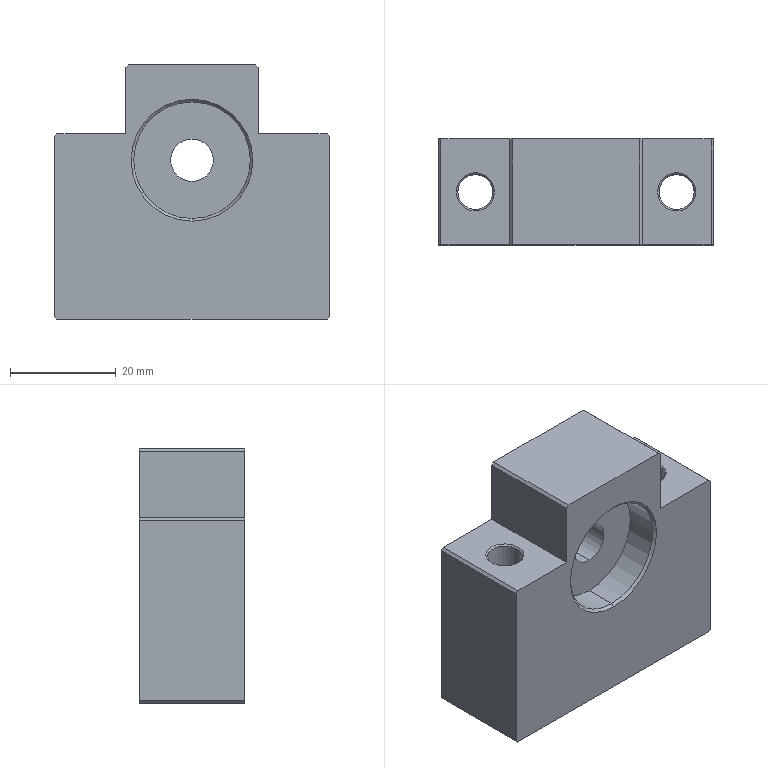Part | SolidWorks | features BaseBody 1 | 1 solid | 36 faces | box 52 x 20 x 48 mm | volume 35177 mm3 | plane 18 | cylinder 10 | cone 8 | commonest cylinder face diameters 6.6 x4 22 x4 8 x2
STEP:
#1=CARTESIAN_POINT('',(290.547,1555.464,-1167.57));
#2=VERTEX_POINT('',#1);
#3=CARTESIAN_POINT('',(290.547,1555.464,-1189.57));
#4=VERTEX_POINT('',#3);
#5=CARTESIAN_POINT('',(290.547,1555.464,-1178.57));
#6=DIRECTION('',(0.,-1.,0.));
#7=DIRECTION('',(1.,0.,0.));
#8=AXIS2_PLACEMENT_3D('',#5,#6,#7);
#9=CIRCLE('',#8,11.);
#10=EDGE_CURVE('',#2,#4,#9,.T.);
#11=ORIENTED_EDGE('',*,*,#10,.F.);
#12=CARTESIAN_POINT('',(290.547,1554.964,-1167.07));
#13=VERTEX_POINT('',#12);
#14=CARTESIAN_POINT('',(290.547,1554.964,-1167.07));
#15=DIRECTION('',(0.,-0.7071,0.7071));
#16=VECTOR('',#15,1000.);
#17=LINE('',#14,#16);
#18=EDGE_CURVE('',#2,#13,#17,.T.);
#19=ORIENTED_EDGE('',*,*,#18,.T.);
#20=CARTESIAN_POINT('',(290.547,1554.964,-1190.07));
#21=VERTEX_POINT('',#20);
#22=CARTESIAN_POINT('',(290.547,1554.964,-1178.57));
#23=DIRECTION('',(0.,-1.,0.));
#24=DIRECTION('',(0.,0.,-1.));
#25=AXIS2_PLACEMENT_3D('',#22,#23,#24);
#26=CIRCLE('',#25,11.5);
#27=EDGE_CURVE('',#13,#21,#26,.T.);
#28=ORIENTED_EDGE('',*,*,#27,.T.);
#29=CARTESIAN_POINT('',(290.547,1554.964,-1190.07));
#30=DIRECTION('',(0.,-0.7071,-0.7071));
#31=VECTOR('',#30,1000.);
#32=LINE('',#29,#31);
#33=EDGE_CURVE('',#4,#21,#32,.T.);
#34=ORIENTED_EDGE('',*,*,#33,.F.);
#35=EDGE_LOOP('',(#11,#19,#28,#34));
#36=FACE_OUTER_BOUND('',#35,.T.);
#37=CARTESIAN_POINT('',(290.547,1554.964,-1178.57));
#38=DIRECTION('',(0.,-1.,0.));
#39=DIRECTION('',(0.,0.,-1.));
#40=AXIS2_PLACEMENT_3D('',#37,#38,#39);
#41=CONICAL_SURFACE('',#40,11.5,0.7854);
#42=ADVANCED_FACE('',(#36),#41,.F.);
#43=ORIENTED_EDGE('',*,*,#10,.T.);
#44=CARTESIAN_POINT('',(290.547,1561.464,-1189.57));
#45=VERTEX_POINT('',#44);
#46=CARTESIAN_POINT('',(290.547,1574.964,-1189.57));
#47=DIRECTION('',(0.,1.,0.));
#48=VECTOR('',#47,1000.);
#49=LINE('',#46,#48);
#50=EDGE_CURVE('',#4,#45,#49,.T.);
#51=ORIENTED_EDGE('',*,*,#50,.T.);
#52=CARTESIAN_POINT('',(290.547,1561.464,-1167.57));
#53=VERTEX_POINT('',#52);
#54=CARTESIAN_POINT('',(290.547,1561.464,-1178.57));
#55=DIRECTION('',(0.,-1.,0.));
#56=DIRECTION('',(0.,0.,1.));
#57=AXIS2_PLACEMENT_3D('',#54,#55,#56);
#58=CIRCLE('',#57,11.);
#59=EDGE_CURVE('',#53,#45,#58,.T.);
#60=ORIENTED_EDGE('',*,*,#59,.F.);
#61=CARTESIAN_POINT('',(290.547,1574.964,-1167.57));
#62=DIRECTION('',(0.,1.,0.));
#63=VECTOR('',#62,1000.);
#64=LINE('',#61,#63);
#65=EDGE_CURVE('',#2,#53,#64,.T.);
#66=ORIENTED_EDGE('',*,*,#65,.F.);
#67=EDGE_LOOP('',(#43,#51,#60,#66));
#68=FACE_OUTER_BOUND('',#67,.T.);
#69=CARTESIAN_POINT('',(290.547,1574.964,-1178.57));
#70=DIRECTION('',(0.,1.,0.));
#71=DIRECTION('',(0.,0.,1.));
#72=AXIS2_PLACEMENT_3D('',#69,#70,#71);
#73=CYLINDRICAL_SURFACE('',#72,11.);
#74=ADVANCED_FACE('',(#68),#73,.F.);
#75=CARTESIAN_POINT('',(312.847,1564.964,-1173.87));
#76=VERTEX_POINT('',#75);
#77=CARTESIAN_POINT('',(306.247,1564.964,-1173.87));
#78=VERTEX_POINT('',#77);
#79=CARTESIAN_POINT('',(309.547,1564.964,-1173.87));
#80=DIRECTION('',(0.,0.,-1.));
#81=DIRECTION('',(-1.,0.,0.));
#82=AXIS2_PLACEMENT_3D('',#79,#80,#81);
#83=CIRCLE('',#82,3.3);
#84=EDGE_CURVE('',#76,#78,#83,.T.);
#85=ORIENTED_EDGE('',*,*,#84,.F.);
#86=CARTESIAN_POINT('',(312.847,1564.964,-1208.57));
#87=VERTEX_POINT('',#86);
#88=CARTESIAN_POINT('',(312.847,1564.964,-1160.569));
#89=DIRECTION('',(0.,0.,-1.));
#90=VECTOR('',#89,1000.);
#91=LINE('',#88,#90);
#92=EDGE_CURVE('',#76,#87,#91,.T.);
#93=ORIENTED_EDGE('',*,*,#92,.T.);
#94=CARTESIAN_POINT('',(306.247,1564.964,-1208.57));
#95=VERTEX_POINT('',#94);
#96=CARTESIAN_POINT('',(309.547,1564.964,-1208.57));
#97=DIRECTION('',(0.,0.,-1.));
#98=DIRECTION('',(-1.,0.,0.));
#99=AXIS2_PLACEMENT_3D('',#96,#97,#98);
#100=CIRCLE('',#99,3.3);
#101=EDGE_CURVE('',#87,#95,#100,.T.);
#102=ORIENTED_EDGE('',*,*,#101,.T.);
#103=CARTESIAN_POINT('',(306.247,1564.964,-1160.569));
#104=DIRECTION('',(0.,0.,-1.));
#105=VECTOR('',#104,1000.);
#106=LINE('',#103,#105);
#107=EDGE_CURVE('',#78,#95,#106,.T.);
#108=ORIENTED_EDGE('',*,*,#107,.F.);
#109=EDGE_LOOP('',(#85,#93,#102,#108));
#110=FACE_OUTER_BOUND('',#109,.T.);
#111=CARTESIAN_POINT('',(309.547,1564.964,-1160.569));
#112=DIRECTION('',(0.,0.,-1.));
#113=DIRECTION('',(-1.,0.,0.));
#114=AXIS2_PLACEMENT_3D('',#111,#112,#113);
#115=CYLINDRICAL_SURFACE('',#114,3.3);
#116=ADVANCED_FACE('',(#110),#115,.F.);
#117=CARTESIAN_POINT('',(274.847,1564.964,-1173.87));
#118=VERTEX_POINT('',#117);
#119=CARTESIAN_POINT('',(268.247,1564.964,-1173.87));
#120=VERTEX_POINT('',#119);
#121=CARTESIAN_POINT('',(271.547,1564.964,-1173.87));
#122=DIRECTION('',(0.,0.,-1.));
#123=DIRECTION('',(-1.,0.,0.));
#124=AXIS2_PLACEMENT_3D('',#121,#122,#123);
#125=CIRCLE('',#124,3.3);
#126=EDGE_CURVE('',#118,#120,#125,.T.);
#127=ORIENTED_EDGE('',*,*,#126,.F.);
#128=CARTESIAN_POINT('',(274.847,1564.964,-1208.57));
#129=VERTEX_POINT('',#128);
#130=CARTESIAN_POINT('',(274.847,1564.964,-1160.569));
#131=DIRECTION('',(0.,0.,-1.));
#132=VECTOR('',#131,1000.);
#133=LINE('',#130,#132);
#134=EDGE_CURVE('',#118,#129,#133,.T.);
#135=ORIENTED_EDGE('',*,*,#134,.T.);
#136=CARTESIAN_POINT('',(268.247,1564.964,-1208.57));
#137=VERTEX_POINT('',#136);
#138=CARTESIAN_POINT('',(271.547,1564.964,-1208.57));
#139=DIRECTION('',(0.,0.,-1.));
#140=DIRECTION('',(-1.,0.,0.));
#141=AXIS2_PLACEMENT_3D('',#138,#139,#140);
#142=CIRCLE('',#141,3.3);
#143=EDGE_CURVE('',#129,#137,#142,.T.);
#144=ORIENTED_EDGE('',*,*,#143,.T.);
#145=CARTESIAN_POINT('',(268.247,1564.964,-1160.569));
#146=DIRECTION('',(0.,0.,-1.));
#147=VECTOR('',#146,1000.);
#148=LINE('',#145,#147);
#149=EDGE_CURVE('',#120,#137,#148,.T.);
#150=ORIENTED_EDGE('',*,*,#149,.F.);
#151=EDGE_LOOP('',(#127,#135,#144,#150));
#152=FACE_OUTER_BOUND('',#151,.T.);
#153=CARTESIAN_POINT('',(271.547,1564.964,-1160.569));
#154=DIRECTION('',(0.,0.,-1.));
#155=DIRECTION('',(-1.,0.,0.));
#156=AXIS2_PLACEMENT_3D('',#153,#154,#155);
#157=CYLINDRICAL_SURFACE('',#156,3.3);
#158=ADVANCED_FACE('',(#152),#157,.F.);
#159=ORIENTED_EDGE('',*,*,#84,.T.);
#160=CARTESIAN_POINT('',(305.947,1564.964,-1173.57));
#161=VERTEX_POINT('',#160);
#162=CARTESIAN_POINT('',(305.947,1564.964,-1173.57));
#163=DIRECTION('',(-0.7071,0.,0.7071));
#164=VECTOR('',#163,1000.);
#165=LINE('',#162,#164);
#166=EDGE_CURVE('',#78,#161,#165,.T.);
#167=ORIENTED_EDGE('',*,*,#166,.T.);
#168=CARTESIAN_POINT('',(313.147,1564.964,-1173.57));
#169=VERTEX_POINT('',#168);
#170=CARTESIAN_POINT('',(309.547,1564.964,-1173.57));
#171=DIRECTION('',(0.,0.,1.));
#172=DIRECTION('',(1.,0.,0.));
#173=AXIS2_PLACEMENT_3D('',#170,#171,#172);
#174=CIRCLE('',#173,3.6);
#175=EDGE_CURVE('',#161,#169,#174,.T.);
#176=ORIENTED_EDGE('',*,*,#175,.T.);
#177=CARTESIAN_POINT('',(313.147,1564.964,-1173.57));
#178=DIRECTION('',(0.7071,0.,0.7071));
#179=VECTOR('',#178,1000.);
#180=LINE('',#177,#179);
#181=EDGE_CURVE('',#76,#169,#180,.T.);
#182=ORIENTED_EDGE('',*,*,#181,.F.);
#183=EDGE_LOOP('',(#159,#167,#176,#182));
#184=FACE_OUTER_BOUND('',#183,.T.);
#185=CARTESIAN_POINT('',(309.547,1564.964,-1173.57));
#186=DIRECTION('',(0.,0.,1.));
#187=DIRECTION('',(1.,0.,0.));
#188=AXIS2_PLACEMENT_3D('',#185,#186,#187);
#189=CONICAL_SURFACE('',#188,3.6,0.7854);
#190=ADVANCED_FACE('',(#184),#189,.F.);
#191=ORIENTED_EDGE('',*,*,#126,.T.);
#192=CARTESIAN_POINT('',(267.947,1564.964,-1173.57));
#193=VERTEX_POINT('',#192);
#194=CARTESIAN_POINT('',(267.947,1564.964,-1173.57));
#195=DIRECTION('',(-0.7071,0.,0.7071));
#196=VECTOR('',#195,1000.);
#197=LINE('',#194,#196);
#198=EDGE_CURVE('',#120,#193,#197,.T.);
#199=ORIENTED_EDGE('',*,*,#198,.T.);
#200=CARTESIAN_POINT('',(275.147,1564.964,-1173.57));
#201=VERTEX_POINT('',#200);
#202=CARTESIAN_POINT('',(271.547,1564.964,-1173.57));
#203=DIRECTION('',(0.,0.,1.));
#204=DIRECTION('',(1.,0.,0.));
#205=AXIS2_PLACEMENT_3D('',#202,#203,#204);
#206=CIRCLE('',#205,3.6);
#207=EDGE_CURVE('',#193,#201,#206,.T.);
#208=ORIENTED_EDGE('',*,*,#207,.T.);
#209=CARTESIAN_POINT('',(275.147,1564.964,-1173.57));
#210=DIRECTION('',(0.7071,0.,0.7071));
#211=VECTOR('',#210,1000.);
#212=LINE('',#209,#211);
#213=EDGE_CURVE('',#118,#201,#212,.T.);
#214=ORIENTED_EDGE('',*,*,#213,.F.);
#215=EDGE_LOOP('',(#191,#199,#208,#214));
#216=FACE_OUTER_BOUND('',#215,.T.);
#217=CARTESIAN_POINT('',(271.547,1564.964,-1173.57));
#218=DIRECTION('',(0.,0.,1.));
#219=DIRECTION('',(1.,0.,0.));
#220=AXIS2_PLACEMENT_3D('',#217,#218,#219);
#221=CONICAL_SURFACE('',#220,3.6,0.7854);
#222=ADVANCED_FACE('',(#216),#221,.F.);
#223=CARTESIAN_POINT('',(290.547,1574.464,-1189.57));
#224=VERTEX_POINT('',#223);
#225=CARTESIAN_POINT('',(290.547,1574.464,-1167.57));
#226=VERTEX_POINT('',#225);
#227=CARTESIAN_POINT('',(290.547,1574.464,-1178.57));
#228=DIRECTION('',(0.,1.,0.));
#229=DIRECTION('',(-1.,0.,0.));
#230=AXIS2_PLACEMENT_3D('',#227,#228,#229);
#231=CIRCLE('',#230,11.);
#232=EDGE_CURVE('',#224,#226,#231,.T.);
#233=ORIENTED_EDGE('',*,*,#232,.F.);
#234=CARTESIAN_POINT('',(290.547,1574.964,-1190.07));
#235=VERTEX_POINT('',#234);
#236=CARTESIAN_POINT('',(290.547,1574.964,-1190.07));
#237=DIRECTION('',(0.,0.7071,-0.7071));
#238=VECTOR('',#237,1000.);
#239=LINE('',#236,#238);
#240=EDGE_CURVE('',#224,#235,#239,.T.);
#241=ORIENTED_EDGE('',*,*,#240,.T.);
#242=CARTESIAN_POINT('',(290.547,1574.964,-1167.07));
#243=VERTEX_POINT('',#242);
#244=CARTESIAN_POINT('',(290.547,1574.964,-1178.57));
#245=DIRECTION('',(0.,-1.,0.));
#246=DIRECTION('',(0.,0.,1.));
#247=AXIS2_PLACEMENT_3D('',#244,#245,#246);
#248=CIRCLE('',#247,11.5);
#249=EDGE_CURVE('',#243,#235,#248,.T.);
#250=ORIENTED_EDGE('',*,*,#249,.F.);
#251=CARTESIAN_POINT('',(290.547,1574.964,-1167.07));
#252=DIRECTION('',(0.,0.7071,0.7071));
#253=VECTOR('',#252,1000.);
#254=LINE('',#251,#253);
#255=EDGE_CURVE('',#226,#243,#254,.T.);
#256=ORIENTED_EDGE('',*,*,#255,.F.);
#257=EDGE_LOOP('',(#233,#241,#250,#256));
#258=FACE_OUTER_BOUND('',#257,.T.);
#259=CARTESIAN_POINT('',(290.547,1574.964,-1178.57));
#260=DIRECTION('',(0.,1.,0.));
#261=DIRECTION('',(0.,0.,1.));
#262=AXIS2_PLACEMENT_3D('',#259,#260,#261);
#263=CONICAL_SURFACE('',#262,11.5,0.7854);
#264=ADVANCED_FACE('',(#258),#263,.F.);
#265=CARTESIAN_POINT('',(290.547,1561.464,-1182.57));
#266=VERTEX_POINT('',#265);
#267=CARTESIAN_POINT('',(290.547,1561.464,-1174.57));
#268=VERTEX_POINT('',#267);
#269=CARTESIAN_POINT('',(290.547,1561.464,-1178.57));
#270=DIRECTION('',(0.,1.,0.));
#271=DIRECTION('',(0.,0.,1.));
#272=AXIS2_PLACEMENT_3D('',#269,#270,#271);
#273=CIRCLE('',#272,4.);
#274=EDGE_CURVE('',#266,#268,#273,.T.);
#275=ORIENTED_EDGE('',*,*,#274,.F.);
#276=CARTESIAN_POINT('',(290.547,1568.464,-1182.57));
#277=VERTEX_POINT('',#276);
#278=CARTESIAN_POINT('',(290.547,1574.964,-1182.57));
#279=DIRECTION('',(0.,1.,0.));
#280=VECTOR('',#279,1000.);
#281=LINE('',#278,#280);
#282=EDGE_CURVE('',#266,#277,#281,.T.);
#283=ORIENTED_EDGE('',*,*,#282,.T.);
#284=CARTESIAN_POINT('',(290.547,1568.464,-1174.57));
#285=VERTEX_POINT('',#284);
#286=CARTESIAN_POINT('',(290.547,1568.464,-1178.57));
#287=DIRECTION('',(0.,-1.,0.));
#288=DIRECTION('',(0.,0.,1.));
#289=AXIS2_PLACEMENT_3D('',#286,#287,#288);
#290=CIRCLE('',#289,4.);
#291=EDGE_CURVE('',#285,#277,#290,.T.);
#292=ORIENTED_EDGE('',*,*,#291,.F.);
#293=CARTESIAN_POINT('',(290.547,1574.964,-1174.57));
#294=DIRECTION('',(0.,1.,0.));
#295=VECTOR('',#294,1000.);
#296=LINE('',#293,#295);
#297=EDGE_CURVE('',#268,#285,#296,.T.);
#298=ORIENTED_EDGE('',*,*,#297,.F.);
#299=EDGE_LOOP('',(#275,#283,#292,#298));
#300=FACE_OUTER_BOUND('',#299,.T.);
#301=CARTESIAN_POINT('',(290.547,1574.964,-1178.57));
#302=DIRECTION('',(0.,1.,0.));
#303=DIRECTION('',(0.,0.,1.));
#304=AXIS2_PLACEMENT_3D('',#301,#302,#303);
#305=CYLINDRICAL_SURFACE('',#304,4.);
#306=ADVANCED_FACE('',(#300),#305,.F.);
#307=CARTESIAN_POINT('',(290.547,1568.464,-1189.57));
#308=VERTEX_POINT('',#307);
#309=CARTESIAN_POINT('',(290.547,1568.464,-1167.57));
#310=VERTEX_POINT('',#309);
#311=CARTESIAN_POINT('',(290.547,1568.464,-1178.57));
#312=DIRECTION('',(0.,1.,0.));
#313=DIRECTION('',(0.,0.,1.));
#314=AXIS2_PLACEMENT_3D('',#311,#312,#313);
#315=CIRCLE('',#314,11.);
#316=EDGE_CURVE('',#308,#310,#315,.T.);
#317=ORIENTED_EDGE('',*,*,#316,.F.);
#318=CARTESIAN_POINT('',(290.547,1574.964,-1189.57));
#319=DIRECTION('',(0.,1.,0.));
#320=VECTOR('',#319,1000.);
#321=LINE('',#318,#320);
#322=EDGE_CURVE('',#308,#224,#321,.T.);
#323=ORIENTED_EDGE('',*,*,#322,.T.);
#324=ORIENTED_EDGE('',*,*,#232,.T.);
#325=CARTESIAN_POINT('',(290.547,1574.964,-1167.57));
#326=DIRECTION('',(0.,1.,0.));
#327=VECTOR('',#326,1000.);
#328=LINE('',#325,#327);
#329=EDGE_CURVE('',#310,#226,#328,.T.);
#330=ORIENTED_EDGE('',*,*,#329,.F.);
#331=EDGE_LOOP('',(#317,#323,#324,#330));
#332=FACE_OUTER_BOUND('',#331,.T.);
#333=CARTESIAN_POINT('',(290.547,1574.964,-1178.57));
#334=DIRECTION('',(0.,1.,0.));
#335=DIRECTION('',(0.,0.,1.));
#336=AXIS2_PLACEMENT_3D('',#333,#334,#335);
#337=CYLINDRICAL_SURFACE('',#336,11.);
#338=ADVANCED_FACE('',(#332),#337,.F.);
#339=CARTESIAN_POINT('',(290.547,1554.964,-1178.57));
#340=DIRECTION('',(0.,-1.,0.));
#341=DIRECTION('',(0.,0.,-1.));
#342=AXIS2_PLACEMENT_3D('',#339,#340,#341);
#343=CIRCLE('',#342,11.5);
#344=EDGE_CURVE('',#21,#13,#343,.T.);
#345=ORIENTED_EDGE('',*,*,#344,.F.);
#346=ORIENTED_EDGE('',*,*,#27,.F.);
#347=EDGE_LOOP('',(#345,#346));
#348=FACE_BOUND('',#347,.T.);
#349=CARTESIAN_POINT('',(316.047,1554.964,-1208.57));
#350=VERTEX_POINT('',#349);
#351=CARTESIAN_POINT('',(265.047,1554.964,-1208.57));
#352=VERTEX_POINT('',#351);
#353=CARTESIAN_POINT('',(290.547,1554.964,-1208.57));
#354=DIRECTION('',(-1.,0.,0.));
#355=VECTOR('',#354,1000.);
#356=LINE('',#353,#355);
#357=EDGE_CURVE('',#350,#352,#356,.T.);
#358=ORIENTED_EDGE('',*,*,#357,.F.);
#359=CARTESIAN_POINT('',(316.547,1554.964,-1208.07));
#360=VERTEX_POINT('',#359);
#361=CARTESIAN_POINT('',(316.547,1554.964,-1208.07));
#362=DIRECTION('',(-0.7071,0.,-0.7071));
#363=VECTOR('',#362,1000.);
#364=LINE('',#361,#363);
#365=EDGE_CURVE('',#360,#350,#364,.T.);
#366=ORIENTED_EDGE('',*,*,#365,.F.);
#367=CARTESIAN_POINT('',(316.547,1554.964,-1174.07));
#368=VERTEX_POINT('',#367);
#369=CARTESIAN_POINT('',(316.547,1554.964,-1208.57));
#370=DIRECTION('',(0.,0.,-1.));
#371=VECTOR('',#370,1000.);
#372=LINE('',#369,#371);
#373=EDGE_CURVE('',#368,#360,#372,.T.);
#374=ORIENTED_EDGE('',*,*,#373,.F.);
#375=CARTESIAN_POINT('',(316.047,1554.964,-1173.57));
#376=VERTEX_POINT('',#375);
#377=CARTESIAN_POINT('',(316.047,1554.964,-1173.57));
#378=DIRECTION('',(0.7071,0.,-0.7071));
#379=VECTOR('',#378,1000.);
#380=LINE('',#377,#379);
#381=EDGE_CURVE('',#376,#368,#380,.T.);
#382=ORIENTED_EDGE('',*,*,#381,.F.);
#383=CARTESIAN_POINT('',(303.047,1554.964,-1173.57));
#384=VERTEX_POINT('',#383);
#385=CARTESIAN_POINT('',(290.547,1554.964,-1173.57));
#386=DIRECTION('',(1.,0.,0.));
#387=VECTOR('',#386,1000.);
#388=LINE('',#385,#387);
#389=EDGE_CURVE('',#384,#376,#388,.T.);
#390=ORIENTED_EDGE('',*,*,#389,.F.);
#391=CARTESIAN_POINT('',(303.047,1554.964,-1161.07));
#392=VERTEX_POINT('',#391);
#393=CARTESIAN_POINT('',(303.047,1554.964,-1208.57));
#394=DIRECTION('',(0.,0.,-1.));
#395=VECTOR('',#394,1000.);
#396=LINE('',#393,#395);
#397=EDGE_CURVE('',#392,#384,#396,.T.);
#398=ORIENTED_EDGE('',*,*,#397,.F.);
#399=CARTESIAN_POINT('',(302.547,1554.964,-1160.57));
#400=VERTEX_POINT('',#399);
#401=CARTESIAN_POINT('',(302.547,1554.964,-1160.57));
#402=DIRECTION('',(0.7071,0.,-0.7071));
#403=VECTOR('',#402,1000.);
#404=LINE('',#401,#403);
#405=EDGE_CURVE('',#400,#392,#404,.T.);
#406=ORIENTED_EDGE('',*,*,#405,.F.);
#407=CARTESIAN_POINT('',(278.547,1554.964,-1160.57));
#408=VERTEX_POINT('',#407);
#409=CARTESIAN_POINT('',(290.547,1554.964,-1160.57));
#410=DIRECTION('',(1.,0.,0.));
#411=VECTOR('',#410,1000.);
#412=LINE('',#409,#411);
#413=EDGE_CURVE('',#408,#400,#412,.T.);
#414=ORIENTED_EDGE('',*,*,#413,.F.);
#415=CARTESIAN_POINT('',(278.047,1554.964,-1161.07));
#416=VERTEX_POINT('',#415);
#417=CARTESIAN_POINT('',(278.047,1554.964,-1161.07));
#418=DIRECTION('',(0.7071,0.,0.7071));
#419=VECTOR('',#418,1000.);
#420=LINE('',#417,#419);
#421=EDGE_CURVE('',#416,#408,#420,.T.);
#422=ORIENTED_EDGE('',*,*,#421,.F.);
#423=CARTESIAN_POINT('',(278.047,1554.964,-1173.57));
#424=VERTEX_POINT('',#423);
#425=CARTESIAN_POINT('',(278.047,1554.964,-1208.57));
#426=DIRECTION('',(0.,0.,1.));
#427=VECTOR('',#426,1000.);
#428=LINE('',#425,#427);
#429=EDGE_CURVE('',#424,#416,#428,.T.);
#430=ORIENTED_EDGE('',*,*,#429,.F.);
#431=CARTESIAN_POINT('',(265.047,1554.964,-1173.57));
#432=VERTEX_POINT('',#431);
#433=CARTESIAN_POINT('',(290.547,1554.964,-1173.57));
#434=DIRECTION('',(1.,0.,0.));
#435=VECTOR('',#434,1000.);
#436=LINE('',#433,#435);
#437=EDGE_CURVE('',#432,#424,#436,.T.);
#438=ORIENTED_EDGE('',*,*,#437,.F.);
#439=CARTESIAN_POINT('',(264.547,1554.964,-1174.07));
#440=VERTEX_POINT('',#439);
#441=CARTESIAN_POINT('',(264.547,1554.964,-1174.07));
#442=DIRECTION('',(0.7071,0.,0.7071));
#443=VECTOR('',#442,1000.);
#444=LINE('',#441,#443);
#445=EDGE_CURVE('',#440,#432,#444,.T.);
#446=ORIENTED_EDGE('',*,*,#445,.F.);
#447=CARTESIAN_POINT('',(264.547,1554.964,-1208.07));
#448=VERTEX_POINT('',#447);
#449=CARTESIAN_POINT('',(264.547,1554.964,-1208.57));
#450=DIRECTION('',(0.,0.,1.));
#451=VECTOR('',#450,1000.);
#452=LINE('',#449,#451);
#453=EDGE_CURVE('',#448,#440,#452,.T.);
#454=ORIENTED_EDGE('',*,*,#453,.F.);
#455=CARTESIAN_POINT('',(265.047,1554.964,-1208.57));
#456=DIRECTION('',(-0.7071,0.,0.7071));
#457=VECTOR('',#456,1000.);
#458=LINE('',#455,#457);
#459=EDGE_CURVE('',#352,#448,#458,.T.);
#460=ORIENTED_EDGE('',*,*,#459,.F.);
#461=EDGE_LOOP('',(#358,#366,#374,#382,#390,#398,#406,#414,#422,#430,#438,#446,#454,#460));
#462=FACE_OUTER_BOUND('',#461,.T.);
#463=CARTESIAN_POINT('',(290.547,1554.964,-1208.57));
#464=DIRECTION('',(0.,1.,0.));
#465=DIRECTION('',(0.,0.,1.));
#466=AXIS2_PLACEMENT_3D('',#463,#464,#465);
#467=PLANE('',#466);
#468=ADVANCED_FACE('',(#348,#462),#467,.F.);
#469=ORIENTED_EDGE('',*,*,#18,.F.);
#470=CARTESIAN_POINT('',(290.547,1555.464,-1178.57));
#471=DIRECTION('',(0.,-1.,0.));
#472=DIRECTION('',(1.,0.,0.));
#473=AXIS2_PLACEMENT_3D('',#470,#471,#472);
#474=CIRCLE('',#473,11.);
#475=EDGE_CURVE('',#4,#2,#474,.T.);
#476=ORIENTED_EDGE('',*,*,#475,.F.);
#477=ORIENTED_EDGE('',*,*,#33,.T.);
#478=ORIENTED_EDGE('',*,*,#344,.T.);
#479=EDGE_LOOP('',(#469,#476,#477,#478));
#480=FACE_OUTER_BOUND('',#479,.T.);
#481=CARTESIAN_POINT('',(290.547,1554.964,-1178.57));
#482=DIRECTION('',(0.,-1.,0.));
#483=DIRECTION('',(0.,0.,-1.));
#484=AXIS2_PLACEMENT_3D('',#481,#482,#483);
#485=CONICAL_SURFACE('',#484,11.5,0.7854);
#486=ADVANCED_FACE('',(#480),#485,.F.);
#487=CARTESIAN_POINT('',(265.047,1574.964,-1208.57));
#488=VERTEX_POINT('',#487);
#489=CARTESIAN_POINT('',(264.547,1574.964,-1208.07));
#490=VERTEX_POINT('',#489);
#491=CARTESIAN_POINT('',(265.047,1574.964,-1208.57));
#492=DIRECTION('',(-0.7071,0.,0.7071));
#493=VECTOR('',#492,1000.);
#494=LINE('',#491,#493);
#495=EDGE_CURVE('',#488,#490,#494,.T.);
#496=ORIENTED_EDGE('',*,*,#495,.F.);
#497=CARTESIAN_POINT('',(265.047,1554.964,-1208.57));
#498=DIRECTION('',(0.,1.,0.));
#499=VECTOR('',#498,1000.);
#500=LINE('',#497,#499);
#501=EDGE_CURVE('',#352,#488,#500,.T.);
#502=ORIENTED_EDGE('',*,*,#501,.F.);
#503=ORIENTED_EDGE('',*,*,#459,.T.);
#504=CARTESIAN_POINT('',(264.547,1554.964,-1208.07));
#505=DIRECTION('',(0.,-1.,0.));
#506=VECTOR('',#505,1000.);
#507=LINE('',#504,#506);
#508=EDGE_CURVE('',#490,#448,#507,.T.);
#509=ORIENTED_EDGE('',*,*,#508,.F.);
#510=EDGE_LOOP('',(#496,#502,#503,#509));
#511=FACE_OUTER_BOUND('',#510,.T.);
#512=CARTESIAN_POINT('',(265.047,1554.964,-1208.57));
#513=DIRECTION('',(0.7071,0.,0.7071));
#514=DIRECTION('',(0.7071,0.,-0.7071));
#515=AXIS2_PLACEMENT_3D('',#512,#513,#514);
#516=PLANE('',#515);
#517=ADVANCED_FACE('',(#511),#516,.F.);
#518=CARTESIAN_POINT('',(309.547,1564.964,-1208.57));
#519=DIRECTION('',(0.,0.,-1.));
#520=DIRECTION('',(-1.,0.,0.));
#521=AXIS2_PLACEMENT_3D('',#518,#519,#520);
#522=CIRCLE('',#521,3.3);
#523=EDGE_CURVE('',#95,#87,#522,.T.);
#524=ORIENTED_EDGE('',*,*,#523,.F.);
#525=ORIENTED_EDGE('',*,*,#101,.F.);
#526=EDGE_LOOP('',(#524,#525));
#527=FACE_BOUND('',#526,.T.);
#528=CARTESIAN_POINT('',(271.547,1564.964,-1208.57));
#529=DIRECTION('',(0.,0.,-1.));
#530=DIRECTION('',(-1.,0.,0.));
#531=AXIS2_PLACEMENT_3D('',#528,#529,#530);
#532=CIRCLE('',#531,3.3);
#533=EDGE_CURVE('',#137,#129,#532,.T.);
#534=ORIENTED_EDGE('',*,*,#533,.F.);
#535=ORIENTED_EDGE('',*,*,#143,.F.);
#536=EDGE_LOOP('',(#534,#535));
#537=FACE_BOUND('',#536,.T.);
#538=CARTESIAN_POINT('',(316.047,1574.964,-1208.57));
#539=VERTEX_POINT('',#538);
#540=CARTESIAN_POINT('',(264.547,1574.964,-1208.57));
#541=DIRECTION('',(-1.,0.,0.));
#542=VECTOR('',#541,1000.);
#543=LINE('',#540,#542);
#544=EDGE_CURVE('',#539,#488,#543,.T.);
#545=ORIENTED_EDGE('',*,*,#544,.F.);
#546=CARTESIAN_POINT('',(316.047,1554.964,-1208.57));
#547=DIRECTION('',(0.,1.,0.));
#548=VECTOR('',#547,1000.);
#549=LINE('',#546,#548);
#550=EDGE_CURVE('',#350,#539,#549,.T.);
#551=ORIENTED_EDGE('',*,*,#550,.F.);
#552=ORIENTED_EDGE('',*,*,#357,.T.);
#553=ORIENTED_EDGE('',*,*,#501,.T.);
#554=EDGE_LOOP('',(#545,#551,#552,#553));
#555=FACE_OUTER_BOUND('',#554,.T.);
#556=CARTESIAN_POINT('',(264.547,1554.964,-1208.57));
#557=DIRECTION('',(0.,0.,1.));
#558=DIRECTION('',(1.,0.,0.));
#559=AXIS2_PLACEMENT_3D('',#556,#557,#558);
#560=PLANE('',#559);
#561=ADVANCED_FACE('',(#527,#537,#555),#560,.F.);
#562=CARTESIAN_POINT('',(316.547,1574.964,-1208.07));
#563=VERTEX_POINT('',#562);
#564=CARTESIAN_POINT('',(316.547,1574.964,-1208.07));
#565=DIRECTION('',(-0.7071,0.,-0.7071));
#566=VECTOR('',#565,1000.);
#567=LINE('',#564,#566);
#568=EDGE_CURVE('',#563,#539,#567,.T.);
#569=ORIENTED_EDGE('',*,*,#568,.F.);
#570=CARTESIAN_POINT('',(316.547,1554.964,-1208.07));
#571=DIRECTION('',(0.,1.,0.));
#572=VECTOR('',#571,1000.);
#573=LINE('',#570,#572);
#574=EDGE_CURVE('',#360,#563,#573,.T.);
#575=ORIENTED_EDGE('',*,*,#574,.F.);
#576=ORIENTED_EDGE('',*,*,#365,.T.);
#577=ORIENTED_EDGE('',*,*,#550,.T.);
#578=EDGE_LOOP('',(#569,#575,#576,#577));
#579=FACE_OUTER_BOUND('',#578,.T.);
#580=CARTESIAN_POINT('',(316.547,1554.964,-1208.07));
#581=DIRECTION('',(-0.7071,0.,0.7071));
#582=DIRECTION('',(0.7071,0.,0.7071));
#583=AXIS2_PLACEMENT_3D('',#580,#581,#582);
#584=PLANE('',#583);
#585=ADVANCED_FACE('',(#579),#584,.F.);
#586=CARTESIAN_POINT('',(316.547,1574.964,-1174.07));
#587=VERTEX_POINT('',#586);
#588=CARTESIAN_POINT('',(316.547,1574.964,-1208.57));
#589=DIRECTION('',(0.,0.,-1.));
#590=VECTOR('',#589,1000.);
#591=LINE('',#588,#590);
#592=EDGE_CURVE('',#587,#563,#591,.T.);
#593=ORIENTED_EDGE('',*,*,#592,.F.);
#594=CARTESIAN_POINT('',(316.547,1554.964,-1174.07));
#595=DIRECTION('',(0.,1.,0.));
#596=VECTOR('',#595,1000.);
#597=LINE('',#594,#596);
#598=EDGE_CURVE('',#368,#587,#597,.T.);
#599=ORIENTED_EDGE('',*,*,#598,.F.);
#600=ORIENTED_EDGE('',*,*,#373,.T.);
#601=ORIENTED_EDGE('',*,*,#574,.T.);
#602=EDGE_LOOP('',(#593,#599,#600,#601));
#603=FACE_OUTER_BOUND('',#602,.T.);
#604=CARTESIAN_POINT('',(316.547,1554.964,-1208.57));
#605=DIRECTION('',(-1.,0.,0.));
#606=DIRECTION('',(0.,0.,1.));
#607=AXIS2_PLACEMENT_3D('',#604,#605,#606);
#608=PLANE('',#607);
#609=ADVANCED_FACE('',(#603),#608,.F.);
#610=CARTESIAN_POINT('',(316.047,1574.964,-1173.57));
#611=VERTEX_POINT('',#610);
#612=CARTESIAN_POINT('',(316.047,1574.964,-1173.57));
#613=DIRECTION('',(0.7071,0.,-0.7071));
#614=VECTOR('',#613,1000.);
#615=LINE('',#612,#614);
#616=EDGE_CURVE('',#611,#587,#615,.T.);
#617=ORIENTED_EDGE('',*,*,#616,.F.);
#618=CARTESIAN_POINT('',(316.047,1554.964,-1173.57));
#619=DIRECTION('',(0.,1.,0.));
#620=VECTOR('',#619,1000.);
#621=LINE('',#618,#620);
#622=EDGE_CURVE('',#376,#611,#621,.T.);
#623=ORIENTED_EDGE('',*,*,#622,.F.);
#624=ORIENTED_EDGE('',*,*,#381,.T.);
#625=ORIENTED_EDGE('',*,*,#598,.T.);
#626=EDGE_LOOP('',(#617,#623,#624,#625));
#627=FACE_OUTER_BOUND('',#626,.T.);
#628=CARTESIAN_POINT('',(316.047,1554.964,-1173.57));
#629=DIRECTION('',(-0.7071,0.,-0.7071));
#630=DIRECTION('',(-0.7071,0.,0.7071));
#631=AXIS2_PLACEMENT_3D('',#628,#629,#630);
#632=PLANE('',#631);
#633=ADVANCED_FACE('',(#627),#632,.F.);
#634=CARTESIAN_POINT('',(309.547,1564.964,-1173.57));
#635=DIRECTION('',(0.,0.,1.));
#636=DIRECTION('',(1.,0.,0.));
#637=AXIS2_PLACEMENT_3D('',#634,#635,#636);
#638=CIRCLE('',#637,3.6);
#639=EDGE_CURVE('',#169,#161,#638,.T.);
#640=ORIENTED_EDGE('',*,*,#639,.F.);
#641=ORIENTED_EDGE('',*,*,#175,.F.);
#642=EDGE_LOOP('',(#640,#641));
#643=FACE_BOUND('',#642,.T.);
#644=CARTESIAN_POINT('',(303.047,1574.964,-1173.57));
#645=VERTEX_POINT('',#644);
#646=CARTESIAN_POINT('',(303.047,1574.964,-1173.57));
#647=DIRECTION('',(1.,0.,0.));
#648=VECTOR('',#647,1000.);
#649=LINE('',#646,#648);
#650=EDGE_CURVE('',#645,#611,#649,.T.);
#651=ORIENTED_EDGE('',*,*,#650,.F.);
#652=CARTESIAN_POINT('',(303.047,1554.964,-1173.57));
#653=DIRECTION('',(0.,1.,0.));
#654=VECTOR('',#653,1000.);
#655=LINE('',#652,#654);
#656=EDGE_CURVE('',#384,#645,#655,.T.);
#657=ORIENTED_EDGE('',*,*,#656,.F.);
#658=ORIENTED_EDGE('',*,*,#389,.T.);
#659=ORIENTED_EDGE('',*,*,#622,.T.);
#660=EDGE_LOOP('',(#651,#657,#658,#659));
#661=FACE_OUTER_BOUND('',#660,.T.);
#662=CARTESIAN_POINT('',(303.047,1554.964,-1173.57));
#663=DIRECTION('',(0.,0.,-1.));
#664=DIRECTION('',(-1.,0.,0.));
#665=AXIS2_PLACEMENT_3D('',#662,#663,#664);
#666=PLANE('',#665);
#667=ADVANCED_FACE('',(#643,#661),#666,.F.);
#668=ORIENTED_EDGE('',*,*,#397,.T.);
#669=ORIENTED_EDGE('',*,*,#656,.T.);
#670=CARTESIAN_POINT('',(303.047,1574.964,-1161.07));
#671=VERTEX_POINT('',#670);
#672=CARTESIAN_POINT('',(303.047,1574.964,-1173.57));
#673=DIRECTION('',(0.,0.,-1.));
#674=VECTOR('',#673,1000.);
#675=LINE('',#672,#674);
#676=EDGE_CURVE('',#671,#645,#675,.T.);
#677=ORIENTED_EDGE('',*,*,#676,.F.);
#678=CARTESIAN_POINT('',(303.047,1554.964,-1161.07));
#679=DIRECTION('',(0.,1.,0.));
#680=VECTOR('',#679,1000.);
#681=LINE('',#678,#680);
#682=EDGE_CURVE('',#392,#671,#681,.T.);
#683=ORIENTED_EDGE('',*,*,#682,.F.);
#684=EDGE_LOOP('',(#668,#669,#677,#683));
#685=FACE_OUTER_BOUND('',#684,.T.);
#686=CARTESIAN_POINT('',(303.047,1554.964,-1173.57));
#687=DIRECTION('',(-1.,0.,0.));
#688=DIRECTION('',(0.,0.,1.));
#689=AXIS2_PLACEMENT_3D('',#686,#687,#688);
#690=PLANE('',#689);
#691=ADVANCED_FACE('',(#685),#690,.F.);
#692=CARTESIAN_POINT('',(302.547,1574.964,-1160.57));
#693=VERTEX_POINT('',#692);
#694=CARTESIAN_POINT('',(302.547,1574.964,-1160.57));
#695=DIRECTION('',(0.7071,0.,-0.7071));
#696=VECTOR('',#695,1000.);
#697=LINE('',#694,#696);
#698=EDGE_CURVE('',#693,#671,#697,.T.);
#699=ORIENTED_EDGE('',*,*,#698,.F.);
#700=CARTESIAN_POINT('',(302.547,1554.964,-1160.57));
#701=DIRECTION('',(0.,1.,0.));
#702=VECTOR('',#701,1000.);
#703=LINE('',#700,#702);
#704=EDGE_CURVE('',#400,#693,#703,.T.);
#705=ORIENTED_EDGE('',*,*,#704,.F.);
#706=ORIENTED_EDGE('',*,*,#405,.T.);
#707=ORIENTED_EDGE('',*,*,#682,.T.);
#708=EDGE_LOOP('',(#699,#705,#706,#707));
#709=FACE_OUTER_BOUND('',#708,.T.);
#710=CARTESIAN_POINT('',(302.547,1554.964,-1160.57));
#711=DIRECTION('',(-0.7071,0.,-0.7071));
#712=DIRECTION('',(-0.7071,0.,0.7071));
#713=AXIS2_PLACEMENT_3D('',#710,#711,#712);
#714=PLANE('',#713);
#715=ADVANCED_FACE('',(#709),#714,.F.);
#716=CARTESIAN_POINT('',(278.547,1574.964,-1160.57));
#717=VERTEX_POINT('',#716);
#718=CARTESIAN_POINT('',(278.047,1574.964,-1160.57));
#719=DIRECTION('',(1.,0.,0.));
#720=VECTOR('',#719,1000.);
#721=LINE('',#718,#720);
#722=EDGE_CURVE('',#717,#693,#721,.T.);
#723=ORIENTED_EDGE('',*,*,#722,.F.);
#724=CARTESIAN_POINT('',(278.547,1554.964,-1160.57));
#725=DIRECTION('',(0.,1.,0.));
#726=VECTOR('',#725,1000.);
#727=LINE('',#724,#726);
#728=EDGE_CURVE('',#408,#717,#727,.T.);
#729=ORIENTED_EDGE('',*,*,#728,.F.);
#730=ORIENTED_EDGE('',*,*,#413,.T.);
#731=ORIENTED_EDGE('',*,*,#704,.T.);
#732=EDGE_LOOP('',(#723,#729,#730,#731));
#733=FACE_OUTER_BOUND('',#732,.T.);
#734=CARTESIAN_POINT('',(278.047,1554.964,-1160.57));
#735=DIRECTION('',(0.,0.,-1.));
#736=DIRECTION('',(-1.,0.,0.));
#737=AXIS2_PLACEMENT_3D('',#734,#735,#736);
#738=PLANE('',#737);
#739=ADVANCED_FACE('',(#733),#738,.F.);
#740=CARTESIAN_POINT('',(278.047,1574.964,-1161.07));
#741=VERTEX_POINT('',#740);
#742=CARTESIAN_POINT('',(278.047,1574.964,-1161.07));
#743=DIRECTION('',(0.7071,0.,0.7071));
#744=VECTOR('',#743,1000.);
#745=LINE('',#742,#744);
#746=EDGE_CURVE('',#741,#717,#745,.T.);
#747=ORIENTED_EDGE('',*,*,#746,.F.);
#748=CARTESIAN_POINT('',(278.047,1554.964,-1161.07));
#749=DIRECTION('',(0.,1.,0.));
#750=VECTOR('',#749,1000.);
#751=LINE('',#748,#750);
#752=EDGE_CURVE('',#416,#741,#751,.T.);
#753=ORIENTED_EDGE('',*,*,#752,.F.);
#754=ORIENTED_EDGE('',*,*,#421,.T.);
#755=ORIENTED_EDGE('',*,*,#728,.T.);
#756=EDGE_LOOP('',(#747,#753,#754,#755));
#757=FACE_OUTER_BOUND('',#756,.T.);
#758=CARTESIAN_POINT('',(278.047,1554.964,-1161.07));
#759=DIRECTION('',(0.7071,0.,-0.7071));
#760=DIRECTION('',(-0.7071,0.,-0.7071));
#761=AXIS2_PLACEMENT_3D('',#758,#759,#760);
#762=PLANE('',#761);
#763=ADVANCED_FACE('',(#757),#762,.F.);
#764=CARTESIAN_POINT('',(278.047,1574.964,-1173.57));
#765=VERTEX_POINT('',#764);
#766=CARTESIAN_POINT('',(278.047,1574.964,-1173.57));
#767=DIRECTION('',(0.,0.,1.));
#768=VECTOR('',#767,1000.);
#769=LINE('',#766,#768);
#770=EDGE_CURVE('',#765,#741,#769,.T.);
#771=ORIENTED_EDGE('',*,*,#770,.F.);
#772=CARTESIAN_POINT('',(278.047,1554.964,-1173.57));
#773=DIRECTION('',(0.,1.,0.));
#774=VECTOR('',#773,1000.);
#775=LINE('',#772,#774);
#776=EDGE_CURVE('',#424,#765,#775,.T.);
#777=ORIENTED_EDGE('',*,*,#776,.F.);
#778=ORIENTED_EDGE('',*,*,#429,.T.);
#779=ORIENTED_EDGE('',*,*,#752,.T.);
#780=EDGE_LOOP('',(#771,#777,#778,#779));
#781=FACE_OUTER_BOUND('',#780,.T.);
#782=CARTESIAN_POINT('',(278.047,1554.964,-1173.57));
#783=DIRECTION('',(1.,0.,0.));
#784=DIRECTION('',(0.,0.,-1.));
#785=AXIS2_PLACEMENT_3D('',#782,#783,#784);
#786=PLANE('',#785);
#787=ADVANCED_FACE('',(#781),#786,.F.);
#788=CARTESIAN_POINT('',(271.547,1564.964,-1173.57));
#789=DIRECTION('',(0.,0.,1.));
#790=DIRECTION('',(1.,0.,0.));
#791=AXIS2_PLACEMENT_3D('',#788,#789,#790);
#792=CIRCLE('',#791,3.6);
#793=EDGE_CURVE('',#201,#193,#792,.T.);
#794=ORIENTED_EDGE('',*,*,#793,.F.);
#795=ORIENTED_EDGE('',*,*,#207,.F.);
#796=EDGE_LOOP('',(#794,#795));
#797=FACE_BOUND('',#796,.T.);
#798=ORIENTED_EDGE('',*,*,#437,.T.);
#799=ORIENTED_EDGE('',*,*,#776,.T.);
#800=CARTESIAN_POINT('',(265.047,1574.964,-1173.57));
#801=VERTEX_POINT('',#800);
#802=CARTESIAN_POINT('',(264.547,1574.964,-1173.57));
#803=DIRECTION('',(1.,0.,0.));
#804=VECTOR('',#803,1000.);
#805=LINE('',#802,#804);
#806=EDGE_CURVE('',#801,#765,#805,.T.);
#807=ORIENTED_EDGE('',*,*,#806,.F.);
#808=CARTESIAN_POINT('',(265.047,1554.964,-1173.57));
#809=DIRECTION('',(0.,1.,0.));
#810=VECTOR('',#809,1000.);
#811=LINE('',#808,#810);
#812=EDGE_CURVE('',#432,#801,#811,.T.);
#813=ORIENTED_EDGE('',*,*,#812,.F.);
#814=EDGE_LOOP('',(#798,#799,#807,#813));
#815=FACE_OUTER_BOUND('',#814,.T.);
#816=CARTESIAN_POINT('',(264.547,1554.964,-1173.57));
#817=DIRECTION('',(0.,0.,-1.));
#818=DIRECTION('',(-1.,0.,0.));
#819=AXIS2_PLACEMENT_3D('',#816,#817,#818);
#820=PLANE('',#819);
#821=ADVANCED_FACE('',(#797,#815),#820,.F.);
#822=CARTESIAN_POINT('',(264.547,1574.964,-1174.07));
#823=VERTEX_POINT('',#822);
#824=CARTESIAN_POINT('',(264.547,1574.964,-1174.07));
#825=DIRECTION('',(0.7071,0.,0.7071));
#826=VECTOR('',#825,1000.);
#827=LINE('',#824,#826);
#828=EDGE_CURVE('',#823,#801,#827,.T.);
#829=ORIENTED_EDGE('',*,*,#828,.F.);
#830=CARTESIAN_POINT('',(264.547,1554.964,-1174.07));
#831=DIRECTION('',(0.,1.,0.));
#832=VECTOR('',#831,1000.);
#833=LINE('',#830,#832);
#834=EDGE_CURVE('',#440,#823,#833,.T.);
#835=ORIENTED_EDGE('',*,*,#834,.F.);
#836=ORIENTED_EDGE('',*,*,#445,.T.);
#837=ORIENTED_EDGE('',*,*,#812,.T.);
#838=EDGE_LOOP('',(#829,#835,#836,#837));
#839=FACE_OUTER_BOUND('',#838,.T.);
#840=CARTESIAN_POINT('',(264.547,1554.964,-1174.07));
#841=DIRECTION('',(0.7071,0.,-0.7071));
#842=DIRECTION('',(-0.7071,0.,-0.7071));
#843=AXIS2_PLACEMENT_3D('',#840,#841,#842);
#844=PLANE('',#843);
#845=ADVANCED_FACE('',(#839),#844,.F.);
#846=ORIENTED_EDGE('',*,*,#453,.T.);
#847=ORIENTED_EDGE('',*,*,#834,.T.);
#848=CARTESIAN_POINT('',(264.547,1574.964,-1208.57));
#849=DIRECTION('',(0.,0.,1.));
#850=VECTOR('',#849,1000.);
#851=LINE('',#848,#850);
#852=EDGE_CURVE('',#490,#823,#851,.T.);
#853=ORIENTED_EDGE('',*,*,#852,.F.);
#854=ORIENTED_EDGE('',*,*,#508,.T.);
#855=EDGE_LOOP('',(#846,#847,#853,#854));
#856=FACE_OUTER_BOUND('',#855,.T.);
#857=CARTESIAN_POINT('',(264.547,1554.964,-1208.57));
#858=DIRECTION('',(1.,0.,0.));
#859=DIRECTION('',(0.,0.,-1.));
#860=AXIS2_PLACEMENT_3D('',#857,#858,#859);
#861=PLANE('',#860);
#862=ADVANCED_FACE('',(#856),#861,.F.);
#863=ORIENTED_EDGE('',*,*,#50,.F.);
#864=ORIENTED_EDGE('',*,*,#475,.T.);
#865=ORIENTED_EDGE('',*,*,#65,.T.);
#866=CARTESIAN_POINT('',(290.547,1561.464,-1178.57));
#867=DIRECTION('',(0.,-1.,0.));
#868=DIRECTION('',(0.,0.,1.));
#869=AXIS2_PLACEMENT_3D('',#866,#867,#868);
#870=CIRCLE('',#869,11.);
#871=EDGE_CURVE('',#45,#53,#870,.T.);
#872=ORIENTED_EDGE('',*,*,#871,.F.);
#873=EDGE_LOOP('',(#863,#864,#865,#872));
#874=FACE_OUTER_BOUND('',#873,.T.);
#875=CARTESIAN_POINT('',(290.547,1574.964,-1178.57));
#876=DIRECTION('',(0.,1.,0.));
#877=DIRECTION('',(0.,0.,1.));
#878=AXIS2_PLACEMENT_3D('',#875,#876,#877);
#879=CYLINDRICAL_SURFACE('',#878,11.);
#880=ADVANCED_FACE('',(#874),#879,.F.);
#881=ORIENTED_EDGE('',*,*,#249,.T.);
#882=CARTESIAN_POINT('',(290.547,1574.964,-1178.57));
#883=DIRECTION('',(0.,-1.,0.));
#884=DIRECTION('',(0.,0.,1.));
#885=AXIS2_PLACEMENT_3D('',#882,#883,#884);
#886=CIRCLE('',#885,11.5);
#887=EDGE_CURVE('',#235,#243,#886,.T.);
#888=ORIENTED_EDGE('',*,*,#887,.T.);
#889=EDGE_LOOP('',(#881,#888));
#890=FACE_BOUND('',#889,.T.);
#891=ORIENTED_EDGE('',*,*,#568,.T.);
#892=ORIENTED_EDGE('',*,*,#544,.T.);
#893=ORIENTED_EDGE('',*,*,#495,.T.);
#894=ORIENTED_EDGE('',*,*,#852,.T.);
#895=ORIENTED_EDGE('',*,*,#828,.T.);
#896=ORIENTED_EDGE('',*,*,#806,.T.);
#897=ORIENTED_EDGE('',*,*,#770,.T.);
#898=ORIENTED_EDGE('',*,*,#746,.T.);
#899=ORIENTED_EDGE('',*,*,#722,.T.);
#900=ORIENTED_EDGE('',*,*,#698,.T.);
#901=ORIENTED_EDGE('',*,*,#676,.T.);
#902=ORIENTED_EDGE('',*,*,#650,.T.);
#903=ORIENTED_EDGE('',*,*,#616,.T.);
#904=ORIENTED_EDGE('',*,*,#592,.T.);
#905=EDGE_LOOP('',(#891,#892,#893,#894,#895,#896,#897,#898,#899,#900,#901,#902,#903,#904));
#906=FACE_OUTER_BOUND('',#905,.T.);
#907=CARTESIAN_POINT('',(290.547,1574.964,-1208.57));
#908=DIRECTION('',(0.,1.,0.));
#909=DIRECTION('',(0.,0.,1.));
#910=AXIS2_PLACEMENT_3D('',#907,#908,#909);
#911=PLANE('',#910);
#912=ADVANCED_FACE('',(#890,#906),#911,.T.);
#913=ORIENTED_EDGE('',*,*,#92,.F.);
#914=CARTESIAN_POINT('',(309.547,1564.964,-1173.87));
#915=DIRECTION('',(0.,0.,-1.));
#916=DIRECTION('',(-1.,0.,0.));
#917=AXIS2_PLACEMENT_3D('',#914,#915,#916);
#918=CIRCLE('',#917,3.3);
#919=EDGE_CURVE('',#78,#76,#918,.T.);
#920=ORIENTED_EDGE('',*,*,#919,.F.);
#921=ORIENTED_EDGE('',*,*,#107,.T.);
#922=ORIENTED_EDGE('',*,*,#523,.T.);
#923=EDGE_LOOP('',(#913,#920,#921,#922));
#924=FACE_OUTER_BOUND('',#923,.T.);
#925=CARTESIAN_POINT('',(309.547,1564.964,-1160.569));
#926=DIRECTION('',(0.,0.,-1.));
#927=DIRECTION('',(-1.,0.,0.));
#928=AXIS2_PLACEMENT_3D('',#925,#926,#927);
#929=CYLINDRICAL_SURFACE('',#928,3.3);
#930=ADVANCED_FACE('',(#924),#929,.F.);
#931=ORIENTED_EDGE('',*,*,#134,.F.);
#932=CARTESIAN_POINT('',(271.547,1564.964,-1173.87));
#933=DIRECTION('',(0.,0.,-1.));
#934=DIRECTION('',(-1.,0.,0.));
#935=AXIS2_PLACEMENT_3D('',#932,#933,#934);
#936=CIRCLE('',#935,3.3);
#937=EDGE_CURVE('',#120,#118,#936,.T.);
#938=ORIENTED_EDGE('',*,*,#937,.F.);
#939=ORIENTED_EDGE('',*,*,#149,.T.);
#940=ORIENTED_EDGE('',*,*,#533,.T.);
#941=EDGE_LOOP('',(#931,#938,#939,#940));
#942=FACE_OUTER_BOUND('',#941,.T.);
#943=CARTESIAN_POINT('',(271.547,1564.964,-1160.569));
#944=DIRECTION('',(0.,0.,-1.));
#945=DIRECTION('',(-1.,0.,0.));
#946=AXIS2_PLACEMENT_3D('',#943,#944,#945);
#947=CYLINDRICAL_SURFACE('',#946,3.3);
#948=ADVANCED_FACE('',(#942),#947,.F.);
#949=ORIENTED_EDGE('',*,*,#166,.F.);
#950=ORIENTED_EDGE('',*,*,#919,.T.);
#951=ORIENTED_EDGE('',*,*,#181,.T.);
#952=ORIENTED_EDGE('',*,*,#639,.T.);
#953=EDGE_LOOP('',(#949,#950,#951,#952));
#954=FACE_OUTER_BOUND('',#953,.T.);
#955=CARTESIAN_POINT('',(309.547,1564.964,-1173.57));
#956=DIRECTION('',(0.,0.,1.));
#957=DIRECTION('',(1.,0.,0.));
#958=AXIS2_PLACEMENT_3D('',#955,#956,#957);
#959=CONICAL_SURFACE('',#958,3.6,0.7854);
#960=ADVANCED_FACE('',(#954),#959,.F.);
#961=ORIENTED_EDGE('',*,*,#198,.F.);
#962=ORIENTED_EDGE('',*,*,#937,.T.);
#963=ORIENTED_EDGE('',*,*,#213,.T.);
#964=ORIENTED_EDGE('',*,*,#793,.T.);
#965=EDGE_LOOP('',(#961,#962,#963,#964));
#966=FACE_OUTER_BOUND('',#965,.T.);
#967=CARTESIAN_POINT('',(271.547,1564.964,-1173.57));
#968=DIRECTION('',(0.,0.,1.));
#969=DIRECTION('',(1.,0.,0.));
#970=AXIS2_PLACEMENT_3D('',#967,#968,#969);
#971=CONICAL_SURFACE('',#970,3.6,0.7854);
#972=ADVANCED_FACE('',(#966),#971,.F.);
#973=CARTESIAN_POINT('',(290.547,1561.464,-1178.57));
#974=DIRECTION('',(0.,1.,0.));
#975=DIRECTION('',(0.,0.,1.));
#976=AXIS2_PLACEMENT_3D('',#973,#974,#975);
#977=CIRCLE('',#976,4.);
#978=EDGE_CURVE('',#268,#266,#977,.T.);
#979=ORIENTED_EDGE('',*,*,#978,.T.);
#980=ORIENTED_EDGE('',*,*,#274,.T.);
#981=EDGE_LOOP('',(#979,#980));
#982=FACE_BOUND('',#981,.T.);
#983=ORIENTED_EDGE('',*,*,#59,.T.);
#984=ORIENTED_EDGE('',*,*,#871,.T.);
#985=EDGE_LOOP('',(#983,#984));
#986=FACE_OUTER_BOUND('',#985,.T.);
#987=CARTESIAN_POINT('',(290.547,1561.464,-1174.57));
#988=DIRECTION('',(0.,-1.,0.));
#989=DIRECTION('',(0.,0.,-1.));
#990=AXIS2_PLACEMENT_3D('',#987,#988,#989);
#991=PLANE('',#990);
#992=ADVANCED_FACE('',(#982,#986),#991,.T.);
#993=ORIENTED_EDGE('',*,*,#240,.F.);
#994=CARTESIAN_POINT('',(290.547,1574.464,-1178.57));
#995=DIRECTION('',(0.,1.,0.));
#996=DIRECTION('',(-1.,0.,0.));
#997=AXIS2_PLACEMENT_3D('',#994,#995,#996);
#998=CIRCLE('',#997,11.);
#999=EDGE_CURVE('',#226,#224,#998,.T.);
#1000=ORIENTED_EDGE('',*,*,#999,.F.);
#1001=ORIENTED_EDGE('',*,*,#255,.T.);
#1002=ORIENTED_EDGE('',*,*,#887,.F.);
#1003=EDGE_LOOP('',(#993,#1000,#1001,#1002));
#1004=FACE_OUTER_BOUND('',#1003,.T.);
#1005=CARTESIAN_POINT('',(290.547,1574.964,-1178.57));
#1006=DIRECTION('',(0.,1.,0.));
#1007=DIRECTION('',(0.,0.,1.));
#1008=AXIS2_PLACEMENT_3D('',#1005,#1006,#1007);
#1009=CONICAL_SURFACE('',#1008,11.5,0.7854);
#1010=ADVANCED_FACE('',(#1004),#1009,.F.);
#1011=ORIENTED_EDGE('',*,*,#282,.F.);
#1012=ORIENTED_EDGE('',*,*,#978,.F.);
#1013=ORIENTED_EDGE('',*,*,#297,.T.);
#1014=CARTESIAN_POINT('',(290.547,1568.464,-1178.57));
#1015=DIRECTION('',(0.,-1.,0.));
#1016=DIRECTION('',(0.,0.,1.));
#1017=AXIS2_PLACEMENT_3D('',#1014,#1015,#1016);
#1018=CIRCLE('',#1017,4.);
#1019=EDGE_CURVE('',#277,#285,#1018,.T.);
#1020=ORIENTED_EDGE('',*,*,#1019,.F.);
#1021=EDGE_LOOP('',(#1011,#1012,#1013,#1020));
#1022=FACE_OUTER_BOUND('',#1021,.T.);
#1023=CARTESIAN_POINT('',(290.547,1574.964,-1178.57));
#1024=DIRECTION('',(0.,1.,0.));
#1025=DIRECTION('',(0.,0.,1.));
#1026=AXIS2_PLACEMENT_3D('',#1023,#1024,#1025);
#1027=CYLINDRICAL_SURFACE('',#1026,4.);
#1028=ADVANCED_FACE('',(#1022),#1027,.F.);
#1029=ORIENTED_EDGE('',*,*,#322,.F.);
#1030=CARTESIAN_POINT('',(290.547,1568.464,-1178.57));
#1031=DIRECTION('',(0.,1.,0.));
#1032=DIRECTION('',(0.,0.,1.));
#1033=AXIS2_PLACEMENT_3D('',#1030,#1031,#1032);
#1034=CIRCLE('',#1033,11.);
#1035=EDGE_CURVE('',#310,#308,#1034,.T.);
#1036=ORIENTED_EDGE('',*,*,#1035,.F.);
#1037=ORIENTED_EDGE('',*,*,#329,.T.);
#1038=ORIENTED_EDGE('',*,*,#999,.T.);
#1039=EDGE_LOOP('',(#1029,#1036,#1037,#1038));
#1040=FACE_OUTER_BOUND('',#1039,.T.);
#1041=CARTESIAN_POINT('',(290.547,1574.964,-1178.57));
#1042=DIRECTION('',(0.,1.,0.));
#1043=DIRECTION('',(0.,0.,1.));
#1044=AXIS2_PLACEMENT_3D('',#1041,#1042,#1043);
#1045=CYLINDRICAL_SURFACE('',#1044,11.);
#1046=ADVANCED_FACE('',(#1040),#1045,.F.);
#1047=ORIENTED_EDGE('',*,*,#291,.T.);
#1048=ORIENTED_EDGE('',*,*,#1019,.T.);
#1049=EDGE_LOOP('',(#1047,#1048));
#1050=FACE_BOUND('',#1049,.T.);
#1051=ORIENTED_EDGE('',*,*,#1035,.T.);
#1052=ORIENTED_EDGE('',*,*,#316,.T.);
#1053=EDGE_LOOP('',(#1051,#1052));
#1054=FACE_OUTER_BOUND('',#1053,.T.);
#1055=CARTESIAN_POINT('',(290.547,1568.464,-1167.57));
#1056=DIRECTION('',(0.,1.,0.));
#1057=DIRECTION('',(0.,0.,1.));
#1058=AXIS2_PLACEMENT_3D('',#1055,#1056,#1057);
#1059=PLANE('',#1058);
#1060=ADVANCED_FACE('',(#1050,#1054),#1059,.T.);
#1061=CLOSED_SHELL('',(#42,#74,#116,#158,#190,#222,#264,#306,#338,#468,#486,#517,#561,#585,#609,#633,#667,#691,#715,#739,#763,#787,#821,#845,#862,#880,#912,#930,#948,#960,#972,#992,#1010,#1028,#1046,#1060));
#1062=MANIFOLD_SOLID_BREP('',#1061);
#1063=CARTESIAN_POINT('',(0.,0.,0.));
#1064=DIRECTION('',(0.,0.,1.));
#1065=DIRECTION('',(1.,0.,0.));
#1066=AXIS2_PLACEMENT_3D('',#1063,#1064,#1065);
#1067=(LENGTH_UNIT()NAMED_UNIT(*)SI_UNIT(.MILLI.,.METRE.));
#1068=UNCERTAINTY_MEASURE_WITH_UNIT(LENGTH_MEASURE(0.00001),#1067,'','');
#1069=(NAMED_UNIT(*)PLANE_ANGLE_UNIT()SI_UNIT($,.RADIAN.));
#1070=(NAMED_UNIT(*)SI_UNIT($,.STERADIAN.)SOLID_ANGLE_UNIT());
#1071=(GEOMETRIC_REPRESENTATION_CONTEXT(3)GLOBAL_UNCERTAINTY_ASSIGNED_CONTEXT((#1068))GLOBAL_UNIT_ASSIGNED_CONTEXT((#1067,#1069,#1070))REPRESENTATION_CONTEXT('',''));
#1072=ADVANCED_BREP_SHAPE_REPRESENTATION('',(#1062,#1066),#1071);